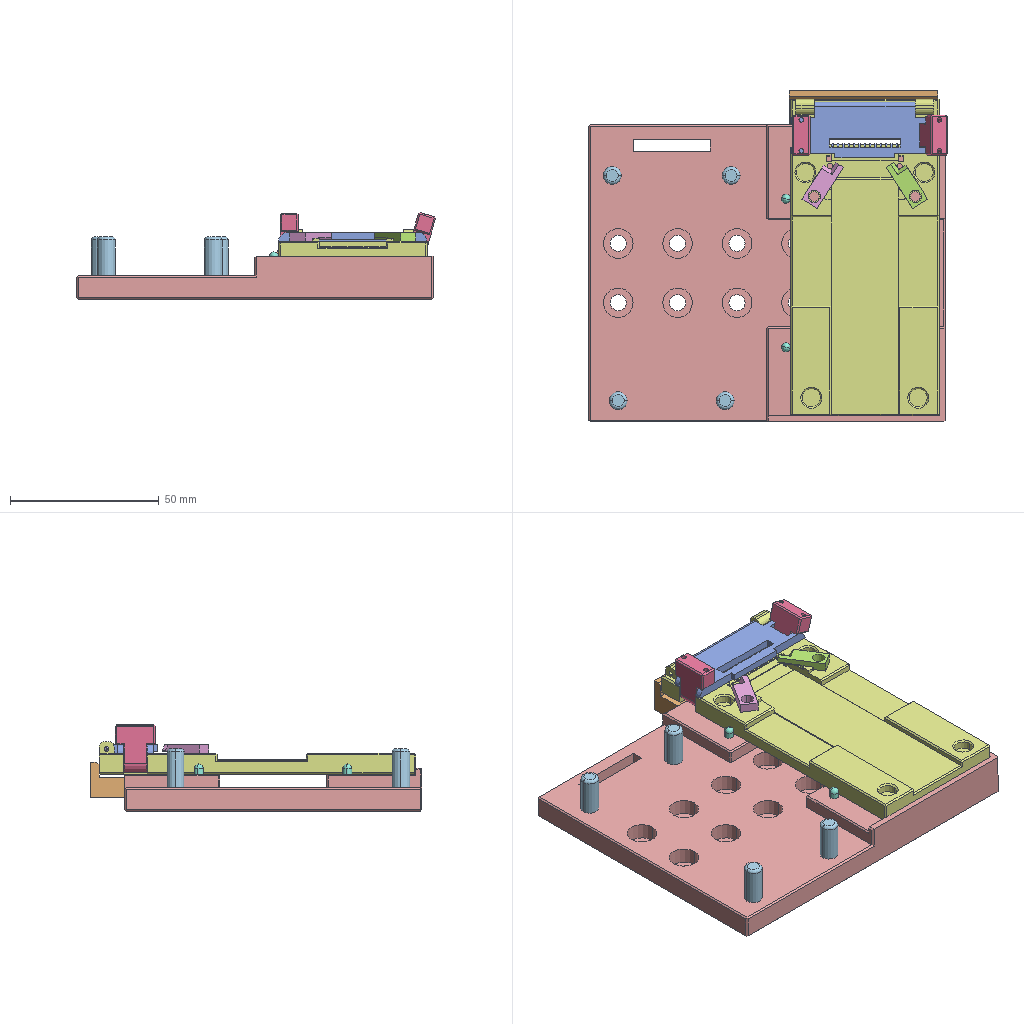Assembly | SolidWorks | 12 different items | 18 placed | box 121 x 112 x 29 mm
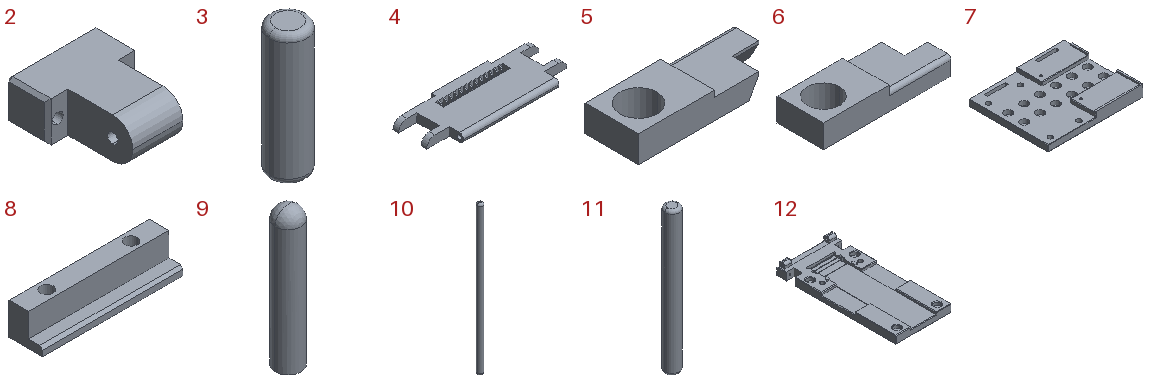Parts list (item | name | quantity | size | volume | features):
1 | (subassembly) | x1 | - | - | -
2 | - | x2 | 13.5 x 16 x 6 mm | 870.216 mm3 | features HoleWzd 2, MirrorPattern 2, Chamfer 1, Extrusion 1, Fillet 1, ICE 1
3 | - | x4 | 6 x 6 x 21 mm | 586.273 mm3 | features Extrusion 1, Fillet 1
4 | - | x1 | 50 x 18.64 x 3.07 mm | 1775 mm3 | features ICE 11, Chamfer 2, Fillet 2, LPattern 2, Extrusion 1, MirrorPattern 1, MoveFace 1
5 | - | x1 | 16.5 x 6 x 3 mm | 192.89 mm3 | features BaseBody 1
6 | - | x1 | 16.5 x 6 x 3 mm | 192.89 mm3 | features BaseBody 1
7 | - | x1 | 120 x 100 x 14.5 mm | 104380 mm3 | features ICE 5, Chamfer 4, LPattern 3, HoleWzd 2, BaseBody 1, Cut 1, DelFace 1, Fillet 1
8 | - | x1 | 50 x 12 x 11.5 mm | 4384 mm3 | features ICE 2, Chamfer 1, Extrusion 1, MoveFace 1
9 | - | x2 | 3 x 3 x 16 mm | 109.563 mm3 | features Extrusion 1, Fillet 1
10 | - | x1 | 1.5 x 1.5 x 40 mm | 70.255 mm3 | features Extrusion 1, Fillet 1
11 | - | x2 | 1.5 x 1.5 x 15 mm | 26.341 mm3 | features Extrusion 1, Fillet 1
12 | - | x1 | - | - | features ICE 11, Chamfer 5, MirrorPattern 3, DelFace 2, Fillet 2, RefSurface 2, BaseBody 1, LPattern 1, MoveFace 1
Mates (type | each side: item.copy, entity, surface, feature):
Coincident | 12.1 face plane Input1 | assembly face
DistanceDim | 12.1 face plane Input1 | assembly face | 2 times
Coincident | 12.1 face plane Input1 | 6.1 face plane Input1
Coincident | 12.1 face plane Input1 | 5.1 face plane Input1
Concentric | 12.1 face cylinder Input1 | 5.1 face cylinder Input1
Concentric | 12.1 face cylinder Input1 | 6.1 face cylinder Input1
Coincident | 12.1 face plane Input1 | 7.1 face plane Input1 | 3 times
Concentric | 7.1 face cylinder Cut-Extrude1 | 9.1 face cylinder Boss-Extrude1
Coincident | 7.1 face plane Input1 | 9.1 face plane Boss-Extrude1
Concentric | 7.1 face cylinder Cut-Extrude1 | 9.2 face cylinder Boss-Extrude1
Coincident | 7.1 face plane Input1 | 9.2 face plane Boss-Extrude1
Coincident | 7.1 face plane Input1 | 8.1 face plane Boss-Extrude1
Concentric | 7.1 face cylinder M4 Tapped Hole1 | 8.1 face cylinder Cut-Extrude1
Concentric | 7.1 face cylinder LPattern1 | 8.1 face cylinder Cut-Extrude1
LimitPlanarAngleDim | 12.1 face plane Boss-Extrude2 | 6.1 face plane Input1
LimitPlanarAngleDim | 5.1 face plane Input1 | 12.1 face plane Boss-Extrude2
Concentric | 12.1 face cylinder Cut-Extrude2 | 4.1 face cylinder Cut-Extrude8
Coincident | 12.1 face plane Boss-Extrude6 | 4.1 face plane Cut-Extrude7
Concentric | 12.1 face cylinder Cut-Extrude2 | 10.1 face cylinder Boss-Extrude1
DistanceDim | 10.1 face plane Boss-Extrude1 | 12.1 face plane Boss-Extrude6
Concentric | 12.1 face cylinder Cut-Extrude5 | 11.1 face cylinder Boss-Extrude1
DistanceDim | 11.1 face plane Boss-Extrude1 | 12.1 face plane Boss-Extrude6
Concentric | 12.1 face cylinder Mirror4 | 11.2 face cylinder Boss-Extrude1
DistanceDim | 11.2 face plane Boss-Extrude1 | 12.1 face plane Boss-Extrude6
Coincident | 12.1 face plane Input1 | 4.1 face plane Boss-Extrude1
Concentric | 11.1 face cylinder Boss-Extrude1 | 2.1 face cylinder Ø1.5 (1.5) Diameter Hole1
Width | 12.1 face plane Cut-Extrude4 | 12.1 face plane Cut-Extrude4 | 2.1 face plane Boss-Extrude1 | 2.1 face plane Boss-Extrude1
Width | 12.1 face plane Mirror3 | 12.1 face plane Mirror3 | 2.2 face plane Boss-Extrude1 | 2.2 face plane Boss-Extrude1
Concentric | 11.2 face cylinder Boss-Extrude1 | 2.2 face cylinder Ø1.5 (1.5) Diameter Hole1
Concentric | 7.1 face cylinder Cut-Extrude10 | 3.1 face cylinder Boss-Extrude1
Concentric | 7.1 face cylinder Cut-Extrude10 | 3.2 face cylinder Boss-Extrude1
Concentric | 7.1 face cylinder Cut-Extrude10 | 3.3 face cylinder Boss-Extrude1
Concentric | 7.1 face cylinder Cut-Extrude10 | 3.4 face cylinder Boss-Extrude1
Coincident | 7.1 face plane Input1 | 3.1 face plane Boss-Extrude1
Coincident | 7.1 face plane Input1 | 3.2 face plane Boss-Extrude1
Coincident | 7.1 face plane Input1 | 3.4 face plane Boss-Extrude1
Coincident | 7.1 face plane Input1 | 3.3 face plane Boss-Extrude1